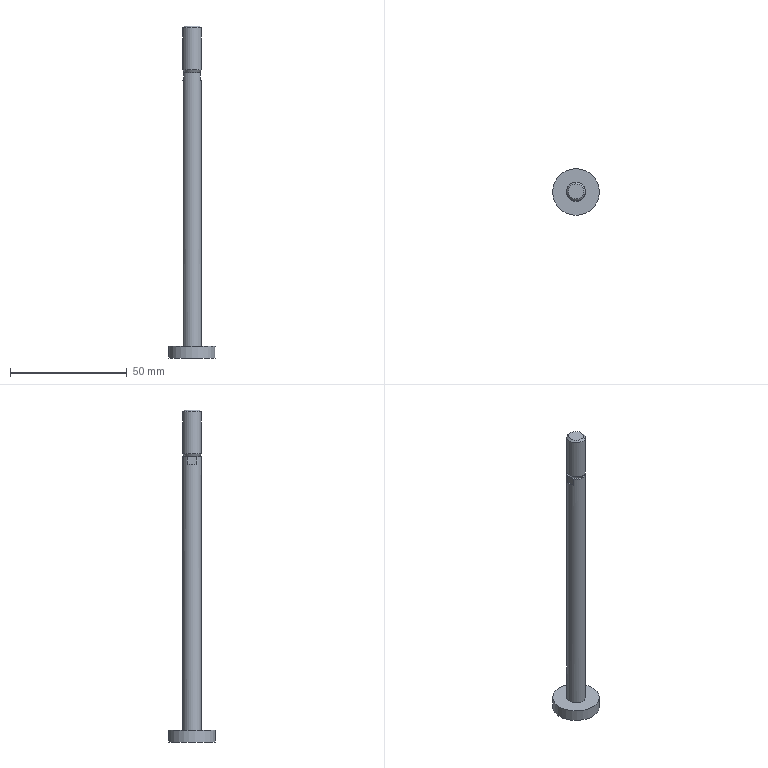Part | STEP file | 1 solid | 13 faces | box 20 x 20 x 142 mm | volume 8430 mm3 | plane 8 | cylinder 3 | cone 2 | commonest cylinder face diameters 8 x2 20 x1
STEP:
#1=CARTESIAN_POINT('',(0.,0.,0.));
#2=DIRECTION('',(0.,0.,1.));
#3=DIRECTION('',(1.,0.,0.));
#4=AXIS2_PLACEMENT_3D('',#1,#2,#3);
#5=CARTESIAN_POINT('',(0.,-3.233,44.));
#6=VERTEX_POINT('',#5);
#7=CARTESIAN_POINT('',(0.,0.,44.));
#8=DIRECTION('',(0.,0.,-1.));
#9=DIRECTION('',(1.,0.,0.));
#10=AXIS2_PLACEMENT_3D('',#7,#8,#9);
#11=CIRCLE('',#10,3.233);
#12=CARTESIAN_POINT('',(0.,0.,43.617));
#13=DIRECTION('',(0.,0.,-1.));
#14=DIRECTION('',(0.,-1.,0.));
#15=AXIS2_PLACEMENT_3D('',#12,#13,#14);
#16=CONICAL_SURFACE('',#15,3.616,0.7854);
#17=CARTESIAN_POINT('',(-1.571,-0.3835));
#18=DIRECTION('',(1.,0.));
#19=VECTOR('',#18,1.);
#20=LINE('',#17,#19);
#21=(GEOMETRIC_REPRESENTATION_CONTEXT(2)PARAMETRIC_REPRESENTATION_CONTEXT()REPRESENTATION_CONTEXT('',''));
#22=DEFINITIONAL_REPRESENTATION('',(#20),#21);
#23=PCURVE('',#16,#22);
#24=CARTESIAN_POINT('',(0.,1.617,44.));
#25=DIRECTION('',(0.,0.,1.));
#26=DIRECTION('',(1.,0.,0.));
#27=AXIS2_PLACEMENT_3D('',#24,#25,#26);
#28=PLANE('',#27);
#29=CARTESIAN_POINT('',(3.233,-1.617));
#30=CARTESIAN_POINT('',(3.233,-7.216));
#31=CARTESIAN_POINT('',(-1.617,-4.416));
#32=CARTESIAN_POINT('',(-6.466,-1.617));
#33=CARTESIAN_POINT('',(-1.617,1.183));
#34=CARTESIAN_POINT('',(3.233,3.983));
#35=CARTESIAN_POINT('',(3.233,-1.617));
#36=(BOUNDED_CURVE()B_SPLINE_CURVE(2,(#29,#30,#31,#32,#33,#34,#35),.UNSPECIFIED.,.T.,.F.)B_SPLINE_CURVE_WITH_KNOTS((1,2,2,2,2,1),(-2.094,0.,2.094,4.189,6.283,8.378),.UNSPECIFIED.)CURVE()GEOMETRIC_REPRESENTATION_ITEM()RATIONAL_B_SPLINE_CURVE((1.,0.5,1.,0.5,1.,0.5,1.))REPRESENTATION_ITEM(''));
#37=(GEOMETRIC_REPRESENTATION_CONTEXT(2)PARAMETRIC_REPRESENTATION_CONTEXT()REPRESENTATION_CONTEXT('',''));
#38=DEFINITIONAL_REPRESENTATION('',(#36),#37);
#39=PCURVE('',#28,#38);
#40=SURFACE_CURVE('',#11,(#23,#39),.PCURVE_S1.);
#41=EDGE_CURVE('',#6,#6,#40,.T.);
#42=ORIENTED_EDGE('',*,*,#41,.T.);
#43=CARTESIAN_POINT('',(0.,-4.,43.233));
#44=VERTEX_POINT('',#43);
#45=CARTESIAN_POINT('',(0.,-3.233,44.));
#46=CARTESIAN_POINT('',(0.,-4.,43.233));
#47=B_SPLINE_CURVE_WITH_KNOTS('',1,(#45,#46),.UNSPECIFIED.,.F.,.F.,(2,2),(-0.5424,0.5424),.PIECEWISE_BEZIER_KNOTS.);
#48=CARTESIAN_POINT('',(6.283,0.));
#49=DIRECTION('',(0.,1.));
#50=VECTOR('',#49,1.);
#51=LINE('',#48,#50);
#52=(GEOMETRIC_REPRESENTATION_CONTEXT(2)PARAMETRIC_REPRESENTATION_CONTEXT()REPRESENTATION_CONTEXT('',''));
#53=DEFINITIONAL_REPRESENTATION('',(#51),#52);
#54=PCURVE('',#16,#53);
#55=CARTESIAN_POINT('',(0.,0.));
#56=DIRECTION('',(0.,1.));
#57=VECTOR('',#56,1.);
#58=LINE('',#55,#57);
#59=(GEOMETRIC_REPRESENTATION_CONTEXT(2)PARAMETRIC_REPRESENTATION_CONTEXT()REPRESENTATION_CONTEXT('',''));
#60=DEFINITIONAL_REPRESENTATION('',(#58),#59);
#61=PCURVE('',#16,#60);
#62=SEAM_CURVE('',#47,(#54,#61),.PCURVE_S1.);
#63=EDGE_CURVE('',#6,#44,#62,.T.);
#64=ORIENTED_EDGE('',*,*,#63,.T.);
#65=CARTESIAN_POINT('',(0.,0.,43.233));
#66=DIRECTION('',(0.,0.,-1.));
#67=DIRECTION('',(1.,0.,0.));
#68=AXIS2_PLACEMENT_3D('',#65,#66,#67);
#69=CIRCLE('',#68,4.);
#70=CARTESIAN_POINT('',(-1.571,0.3835));
#71=DIRECTION('',(1.,0.));
#72=VECTOR('',#71,1.);
#73=LINE('',#70,#72);
#74=(GEOMETRIC_REPRESENTATION_CONTEXT(2)PARAMETRIC_REPRESENTATION_CONTEXT()REPRESENTATION_CONTEXT('',''));
#75=DEFINITIONAL_REPRESENTATION('',(#73),#74);
#76=PCURVE('',#16,#75);
#77=CARTESIAN_POINT('',(0.,0.,34.281));
#78=DIRECTION('',(0.,0.,-1.));
#79=DIRECTION('',(0.,-1.,0.));
#80=AXIS2_PLACEMENT_3D('',#77,#78,#79);
#81=CYLINDRICAL_SURFACE('',#80,4.);
#82=CARTESIAN_POINT('',(-1.571,-8.952));
#83=DIRECTION('',(1.,0.));
#84=VECTOR('',#83,1.);
#85=LINE('',#82,#84);
#86=(GEOMETRIC_REPRESENTATION_CONTEXT(2)PARAMETRIC_REPRESENTATION_CONTEXT()REPRESENTATION_CONTEXT('',''));
#87=DEFINITIONAL_REPRESENTATION('',(#85),#86);
#88=PCURVE('',#81,#87);
#89=SURFACE_CURVE('',#69,(#76,#88),.PCURVE_S1.);
#90=EDGE_CURVE('',#44,#44,#89,.T.);
#91=ORIENTED_EDGE('',*,*,#90,.F.);
#92=ORIENTED_EDGE('',*,*,#63,.F.);
#93=EDGE_LOOP('',(#42,#64,#91,#92));
#94=FACE_BOUND('',#93,.T.);
#95=ADVANCED_FACE('',(#94),#16,.T.);
#96=ORIENTED_EDGE('',*,*,#90,.T.);
#97=CARTESIAN_POINT('',(0.,-4.,25.328));
#98=VERTEX_POINT('',#97);
#99=CARTESIAN_POINT('',(0.,-4.,43.233));
#100=CARTESIAN_POINT('',(0.,-4.,25.328));
#101=B_SPLINE_CURVE_WITH_KNOTS('',1,(#99,#100),.UNSPECIFIED.,.F.,.F.,(2,2),(-8.952,8.952),.PIECEWISE_BEZIER_KNOTS.);
#102=CARTESIAN_POINT('',(6.283,0.));
#103=DIRECTION('',(0.,1.));
#104=VECTOR('',#103,1.);
#105=LINE('',#102,#104);
#106=(GEOMETRIC_REPRESENTATION_CONTEXT(2)PARAMETRIC_REPRESENTATION_CONTEXT()REPRESENTATION_CONTEXT('',''));
#107=DEFINITIONAL_REPRESENTATION('',(#105),#106);
#108=PCURVE('',#81,#107);
#109=CARTESIAN_POINT('',(0.,0.));
#110=DIRECTION('',(0.,1.));
#111=VECTOR('',#110,1.);
#112=LINE('',#109,#111);
#113=(GEOMETRIC_REPRESENTATION_CONTEXT(2)PARAMETRIC_REPRESENTATION_CONTEXT()REPRESENTATION_CONTEXT('',''));
#114=DEFINITIONAL_REPRESENTATION('',(#112),#113);
#115=PCURVE('',#81,#114);
#116=SEAM_CURVE('',#101,(#108,#115),.PCURVE_S1.);
#117=EDGE_CURVE('',#44,#98,#116,.T.);
#118=ORIENTED_EDGE('',*,*,#117,.T.);
#119=CARTESIAN_POINT('',(0.,0.,25.328));
#120=DIRECTION('',(0.,0.,1.));
#121=DIRECTION('',(0.,-1.,0.));
#122=AXIS2_PLACEMENT_3D('',#119,#120,#121);
#123=CIRCLE('',#122,4.);
#124=CARTESIAN_POINT('',(6.283,8.952));
#125=DIRECTION('',(-1.,0.));
#126=VECTOR('',#125,1.);
#127=LINE('',#124,#126);
#128=(GEOMETRIC_REPRESENTATION_CONTEXT(2)PARAMETRIC_REPRESENTATION_CONTEXT()REPRESENTATION_CONTEXT('',''));
#129=DEFINITIONAL_REPRESENTATION('',(#127),#128);
#130=PCURVE('',#81,#129);
#131=CARTESIAN_POINT('',(0.,0.,24.664));
#132=DIRECTION('',(0.,0.,1.));
#133=DIRECTION('',(0.,1.,0.));
#134=AXIS2_PLACEMENT_3D('',#131,#132,#133);
#135=CONICAL_SURFACE('',#134,3.616,0.5236);
#136=CARTESIAN_POINT('',(3.142,0.6642));
#137=DIRECTION('',(1.,0.));
#138=VECTOR('',#137,1.);
#139=LINE('',#136,#138);
#140=(GEOMETRIC_REPRESENTATION_CONTEXT(2)PARAMETRIC_REPRESENTATION_CONTEXT()REPRESENTATION_CONTEXT('',''));
#141=DEFINITIONAL_REPRESENTATION('',(#139),#140);
#142=PCURVE('',#135,#141);
#143=SURFACE_CURVE('',#123,(#130,#142),.PCURVE_S1.);
#144=EDGE_CURVE('',#98,#98,#143,.T.);
#145=ORIENTED_EDGE('',*,*,#144,.T.);
#146=ORIENTED_EDGE('',*,*,#117,.F.);
#147=EDGE_LOOP('',(#96,#118,#145,#146));
#148=FACE_BOUND('',#147,.T.);
#149=ADVANCED_FACE('',(#148),#81,.T.);
#150=ORIENTED_EDGE('',*,*,#41,.F.);
#151=EDGE_LOOP('',(#150));
#152=FACE_BOUND('',#151,.T.);
#153=ADVANCED_FACE('',(#152),#28,.T.);
#154=ORIENTED_EDGE('',*,*,#144,.F.);
#155=CARTESIAN_POINT('',(0.,-3.233,24.));
#156=VERTEX_POINT('',#155);
#157=CARTESIAN_POINT('',(0.,-3.233,24.));
#158=CARTESIAN_POINT('',(0.,-4.,25.328));
#159=B_SPLINE_CURVE_WITH_KNOTS('',1,(#157,#158),.UNSPECIFIED.,.F.,.F.,(2,2),(-0.767,0.767),.PIECEWISE_BEZIER_KNOTS.);
#160=CARTESIAN_POINT('',(3.142,0.));
#161=DIRECTION('',(0.,1.));
#162=VECTOR('',#161,1.);
#163=LINE('',#160,#162);
#164=(GEOMETRIC_REPRESENTATION_CONTEXT(2)PARAMETRIC_REPRESENTATION_CONTEXT()REPRESENTATION_CONTEXT('',''));
#165=DEFINITIONAL_REPRESENTATION('',(#163),#164);
#166=PCURVE('',#135,#165);
#167=CARTESIAN_POINT('',(9.425,0.));
#168=DIRECTION('',(0.,1.));
#169=VECTOR('',#168,1.);
#170=LINE('',#167,#169);
#171=(GEOMETRIC_REPRESENTATION_CONTEXT(2)PARAMETRIC_REPRESENTATION_CONTEXT()REPRESENTATION_CONTEXT('',''));
#172=DEFINITIONAL_REPRESENTATION('',(#170),#171);
#173=PCURVE('',#135,#172);
#174=SEAM_CURVE('',#159,(#166,#173),.PCURVE_S1.);
#175=EDGE_CURVE('',#156,#98,#174,.T.);
#176=ORIENTED_EDGE('',*,*,#175,.F.);
#177=CARTESIAN_POINT('',(0.,0.,24.));
#178=DIRECTION('',(0.,0.,1.));
#179=DIRECTION('',(1.,0.,0.));
#180=AXIS2_PLACEMENT_3D('',#177,#178,#179);
#181=CIRCLE('',#180,3.233);
#182=CARTESIAN_POINT('',(-1.571,-0.6642));
#183=DIRECTION('',(1.,0.));
#184=VECTOR('',#183,1.);
#185=LINE('',#182,#184);
#186=(GEOMETRIC_REPRESENTATION_CONTEXT(2)PARAMETRIC_REPRESENTATION_CONTEXT()REPRESENTATION_CONTEXT('',''));
#187=DEFINITIONAL_REPRESENTATION('',(#185),#186);
#188=PCURVE('',#135,#187);
#189=CARTESIAN_POINT('',(0.,3.616,24.));
#190=DIRECTION('',(0.,0.,1.));
#191=DIRECTION('',(1.,0.,0.));
#192=AXIS2_PLACEMENT_3D('',#189,#190,#191);
#193=PLANE('',#192);
#194=CARTESIAN_POINT('',(0.,-3.616));
#195=DIRECTION('',(1.,0.));
#196=AXIS2_PLACEMENT_2D('',#194,#195);
#197=CIRCLE('',#196,3.233);
#198=(GEOMETRIC_REPRESENTATION_CONTEXT(2)PARAMETRIC_REPRESENTATION_CONTEXT()REPRESENTATION_CONTEXT('',''));
#199=DEFINITIONAL_REPRESENTATION('',(#197),#198);
#200=PCURVE('',#193,#199);
#201=SURFACE_CURVE('',#181,(#188,#200),.PCURVE_S1.);
#202=EDGE_CURVE('',#156,#156,#201,.T.);
#203=ORIENTED_EDGE('',*,*,#202,.T.);
#204=ORIENTED_EDGE('',*,*,#175,.T.);
#205=EDGE_LOOP('',(#154,#176,#203,#204));
#206=FACE_BOUND('',#205,.T.);
#207=ADVANCED_FACE('',(#206),#135,.T.);
#208=CARTESIAN_POINT('',(-3.5,1.936,24.));
#209=VERTEX_POINT('',#208);
#210=CARTESIAN_POINT('',(-3.5,-1.936,24.));
#211=VERTEX_POINT('',#210);
#212=CARTESIAN_POINT('',(-3.5,1.936,24.));
#213=DIRECTION('',(0.,-1.,0.));
#214=VECTOR('',#213,1.);
#215=LINE('',#212,#214);
#216=CARTESIAN_POINT('',(-3.5,-1.68));
#217=DIRECTION('',(0.,-1.));
#218=VECTOR('',#217,1.);
#219=LINE('',#216,#218);
#220=(GEOMETRIC_REPRESENTATION_CONTEXT(2)PARAMETRIC_REPRESENTATION_CONTEXT()REPRESENTATION_CONTEXT('',''));
#221=DEFINITIONAL_REPRESENTATION('',(#219),#220);
#222=PCURVE('',#193,#221);
#223=CARTESIAN_POINT('',(-3.5,20.,24.));
#224=DIRECTION('',(1.,0.,0.));
#225=DIRECTION('',(0.,0.,-1.));
#226=AXIS2_PLACEMENT_3D('',#223,#224,#225);
#227=PLANE('',#226);
#228=CARTESIAN_POINT('',(0.,-18.064));
#229=DIRECTION('',(0.,-1.));
#230=VECTOR('',#229,1.);
#231=LINE('',#228,#230);
#232=(GEOMETRIC_REPRESENTATION_CONTEXT(2)PARAMETRIC_REPRESENTATION_CONTEXT()REPRESENTATION_CONTEXT('',''));
#233=DEFINITIONAL_REPRESENTATION('',(#231),#232);
#234=PCURVE('',#227,#233);
#235=SURFACE_CURVE('',#215,(#222,#234),.PCURVE_S1.);
#236=EDGE_CURVE('',#209,#211,#235,.T.);
#237=ORIENTED_EDGE('',*,*,#236,.T.);
#238=CARTESIAN_POINT('',(0.,-4.,24.));
#239=VERTEX_POINT('',#238);
#240=CARTESIAN_POINT('',(-0.000000002,-0.000000003,24.));
#241=DIRECTION('',(0.,0.,1.));
#242=DIRECTION('',(1.,0.,0.));
#243=AXIS2_PLACEMENT_3D('',#240,#241,#242);
#244=CIRCLE('',#243,4.);
#245=CARTESIAN_POINT('',(-0.000000002,-3.617));
#246=DIRECTION('',(1.,0.));
#247=AXIS2_PLACEMENT_2D('',#245,#246);
#248=CIRCLE('',#247,4.);
#249=(GEOMETRIC_REPRESENTATION_CONTEXT(2)PARAMETRIC_REPRESENTATION_CONTEXT()REPRESENTATION_CONTEXT('',''));
#250=DEFINITIONAL_REPRESENTATION('',(#248),#249);
#251=PCURVE('',#193,#250);
#252=CARTESIAN_POINT('',(0.,0.,-34.5));
#253=DIRECTION('',(0.,0.,-1.));
#254=DIRECTION('',(0.,-1.,0.));
#255=AXIS2_PLACEMENT_3D('',#252,#253,#254);
#256=CYLINDRICAL_SURFACE('',#255,4.);
#257=CARTESIAN_POINT('',(1.065,-58.5));
#258=CARTESIAN_POINT('',(-1.065,-58.5));
#259=B_SPLINE_CURVE_WITH_KNOTS('',1,(#257,#258),.UNSPECIFIED.,.F.,.F.,(2,2),(3.647,5.778),.PIECEWISE_BEZIER_KNOTS.);
#260=(GEOMETRIC_REPRESENTATION_CONTEXT(2)PARAMETRIC_REPRESENTATION_CONTEXT()REPRESENTATION_CONTEXT('',''));
#261=DEFINITIONAL_REPRESENTATION('',(#259),#260);
#262=PCURVE('',#256,#261);
#263=SURFACE_CURVE('',#244,(#251,#262),.PCURVE_S1.);
#264=EDGE_CURVE('',#211,#239,#263,.T.);
#265=ORIENTED_EDGE('',*,*,#264,.T.);
#266=CARTESIAN_POINT('',(3.5,-1.936,24.));
#267=VERTEX_POINT('',#266);
#268=CARTESIAN_POINT('',(-0.000000002,-0.000000003,24.));
#269=DIRECTION('',(0.,0.,1.));
#270=DIRECTION('',(1.,0.,0.));
#271=AXIS2_PLACEMENT_3D('',#268,#269,#270);
#272=CIRCLE('',#271,4.);
#273=CARTESIAN_POINT('',(-0.000000002,-3.617));
#274=DIRECTION('',(1.,0.));
#275=AXIS2_PLACEMENT_2D('',#273,#274);
#276=CIRCLE('',#275,4.);
#277=(GEOMETRIC_REPRESENTATION_CONTEXT(2)PARAMETRIC_REPRESENTATION_CONTEXT()REPRESENTATION_CONTEXT('',''));
#278=DEFINITIONAL_REPRESENTATION('',(#276),#277);
#279=PCURVE('',#193,#278);
#280=CARTESIAN_POINT('',(7.349,-58.5));
#281=CARTESIAN_POINT('',(5.218,-58.5));
#282=B_SPLINE_CURVE_WITH_KNOTS('',1,(#280,#281),.UNSPECIFIED.,.F.,.F.,(2,2),(3.647,5.778),.PIECEWISE_BEZIER_KNOTS.);
#283=(GEOMETRIC_REPRESENTATION_CONTEXT(2)PARAMETRIC_REPRESENTATION_CONTEXT()REPRESENTATION_CONTEXT('',''));
#284=DEFINITIONAL_REPRESENTATION('',(#282),#283);
#285=PCURVE('',#256,#284);
#286=SURFACE_CURVE('',#272,(#279,#285),.PCURVE_S1.);
#287=EDGE_CURVE('',#239,#267,#286,.T.);
#288=ORIENTED_EDGE('',*,*,#287,.T.);
#289=CARTESIAN_POINT('',(3.5,1.936,24.));
#290=VERTEX_POINT('',#289);
#291=CARTESIAN_POINT('',(3.5,-1.936,24.));
#292=DIRECTION('',(0.,1.,0.));
#293=VECTOR('',#292,1.);
#294=LINE('',#291,#293);
#295=CARTESIAN_POINT('',(3.5,-5.553));
#296=DIRECTION('',(0.,1.));
#297=VECTOR('',#296,1.);
#298=LINE('',#295,#297);
#299=(GEOMETRIC_REPRESENTATION_CONTEXT(2)PARAMETRIC_REPRESENTATION_CONTEXT()REPRESENTATION_CONTEXT('',''));
#300=DEFINITIONAL_REPRESENTATION('',(#298),#299);
#301=PCURVE('',#193,#300);
#302=CARTESIAN_POINT('',(3.5,20.,20.8));
#303=DIRECTION('',(-1.,0.,0.));
#304=DIRECTION('',(0.,0.,1.));
#305=AXIS2_PLACEMENT_3D('',#302,#303,#304);
#306=PLANE('',#305);
#307=CARTESIAN_POINT('',(3.2,-21.936));
#308=DIRECTION('',(0.,1.));
#309=VECTOR('',#308,1.);
#310=LINE('',#307,#309);
#311=(GEOMETRIC_REPRESENTATION_CONTEXT(2)PARAMETRIC_REPRESENTATION_CONTEXT()REPRESENTATION_CONTEXT('',''));
#312=DEFINITIONAL_REPRESENTATION('',(#310),#311);
#313=PCURVE('',#306,#312);
#314=SURFACE_CURVE('',#294,(#301,#313),.PCURVE_S1.);
#315=EDGE_CURVE('',#267,#290,#314,.T.);
#316=ORIENTED_EDGE('',*,*,#315,.T.);
#317=CARTESIAN_POINT('',(-0.000000003,-0.000000003,24.));
#318=DIRECTION('',(0.,0.,1.));
#319=DIRECTION('',(1.,0.,0.));
#320=AXIS2_PLACEMENT_3D('',#317,#318,#319);
#321=CIRCLE('',#320,4.);
#322=CARTESIAN_POINT('',(-0.000000003,-3.617));
#323=DIRECTION('',(1.,0.));
#324=AXIS2_PLACEMENT_2D('',#322,#323);
#325=CIRCLE('',#324,4.);
#326=(GEOMETRIC_REPRESENTATION_CONTEXT(2)PARAMETRIC_REPRESENTATION_CONTEXT()REPRESENTATION_CONTEXT('',''));
#327=DEFINITIONAL_REPRESENTATION('',(#325),#326);
#328=PCURVE('',#193,#327);
#329=CARTESIAN_POINT('',(4.207,-58.5));
#330=CARTESIAN_POINT('',(2.076,-58.5));
#331=B_SPLINE_CURVE_WITH_KNOTS('',1,(#329,#330),.UNSPECIFIED.,.F.,.F.,(2,2),(0.5054,2.636),.PIECEWISE_BEZIER_KNOTS.);
#332=(GEOMETRIC_REPRESENTATION_CONTEXT(2)PARAMETRIC_REPRESENTATION_CONTEXT()REPRESENTATION_CONTEXT('',''));
#333=DEFINITIONAL_REPRESENTATION('',(#331),#332);
#334=PCURVE('',#256,#333);
#335=SURFACE_CURVE('',#321,(#328,#334),.PCURVE_S1.);
#336=EDGE_CURVE('',#290,#209,#335,.T.);
#337=ORIENTED_EDGE('',*,*,#336,.T.);
#338=EDGE_LOOP('',(#237,#265,#288,#316,#337));
#339=FACE_BOUND('',#338,.T.);
#340=ORIENTED_EDGE('',*,*,#202,.F.);
#341=EDGE_LOOP('',(#340));
#342=FACE_BOUND('',#341,.T.);
#343=ADVANCED_FACE('',(#339,#342),#193,.T.);
#344=CARTESIAN_POINT('',(-3.5,-1.936,20.8));
#345=VERTEX_POINT('',#344);
#346=CARTESIAN_POINT('',(-3.5,-1.936,24.));
#347=DIRECTION('',(0.,0.,-1.));
#348=VECTOR('',#347,1.);
#349=LINE('',#346,#348);
#350=CARTESIAN_POINT('',(0.,-21.936));
#351=DIRECTION('',(1.,0.));
#352=VECTOR('',#351,1.);
#353=LINE('',#350,#352);
#354=(GEOMETRIC_REPRESENTATION_CONTEXT(2)PARAMETRIC_REPRESENTATION_CONTEXT()REPRESENTATION_CONTEXT('',''));
#355=DEFINITIONAL_REPRESENTATION('',(#353),#354);
#356=PCURVE('',#227,#355);
#357=CARTESIAN_POINT('',(1.065,-58.5));
#358=DIRECTION('',(0.,1.));
#359=VECTOR('',#358,1.);
#360=LINE('',#357,#359);
#361=(GEOMETRIC_REPRESENTATION_CONTEXT(2)PARAMETRIC_REPRESENTATION_CONTEXT()REPRESENTATION_CONTEXT('',''));
#362=DEFINITIONAL_REPRESENTATION('',(#360),#361);
#363=PCURVE('',#256,#362);
#364=SURFACE_CURVE('',#349,(#356,#363),.PCURVE_S1.);
#365=EDGE_CURVE('',#211,#345,#364,.T.);
#366=ORIENTED_EDGE('',*,*,#365,.F.);
#367=ORIENTED_EDGE('',*,*,#236,.F.);
#368=CARTESIAN_POINT('',(-3.5,1.936,20.8));
#369=VERTEX_POINT('',#368);
#370=CARTESIAN_POINT('',(-3.5,1.936,20.8));
#371=DIRECTION('',(0.,0.,1.));
#372=VECTOR('',#371,1.);
#373=LINE('',#370,#372);
#374=CARTESIAN_POINT('',(3.2,-18.064));
#375=DIRECTION('',(-1.,0.));
#376=VECTOR('',#375,1.);
#377=LINE('',#374,#376);
#378=(GEOMETRIC_REPRESENTATION_CONTEXT(2)PARAMETRIC_REPRESENTATION_CONTEXT()REPRESENTATION_CONTEXT('',''));
#379=DEFINITIONAL_REPRESENTATION('',(#377),#378);
#380=PCURVE('',#227,#379);
#381=CARTESIAN_POINT('',(2.076,-55.3));
#382=DIRECTION('',(0.,-1.));
#383=VECTOR('',#382,1.);
#384=LINE('',#381,#383);
#385=(GEOMETRIC_REPRESENTATION_CONTEXT(2)PARAMETRIC_REPRESENTATION_CONTEXT()REPRESENTATION_CONTEXT('',''));
#386=DEFINITIONAL_REPRESENTATION('',(#384),#385);
#387=PCURVE('',#256,#386);
#388=SURFACE_CURVE('',#373,(#380,#387),.PCURVE_S1.);
#389=EDGE_CURVE('',#369,#209,#388,.T.);
#390=ORIENTED_EDGE('',*,*,#389,.F.);
#391=CARTESIAN_POINT('',(-3.5,1.936,20.8));
#392=DIRECTION('',(0.,-1.,0.));
#393=VECTOR('',#392,1.);
#394=LINE('',#391,#393);
#395=CARTESIAN_POINT('',(3.2,-18.064));
#396=DIRECTION('',(0.,-1.));
#397=VECTOR('',#396,1.);
#398=LINE('',#395,#397);
#399=(GEOMETRIC_REPRESENTATION_CONTEXT(2)PARAMETRIC_REPRESENTATION_CONTEXT()REPRESENTATION_CONTEXT('',''));
#400=DEFINITIONAL_REPRESENTATION('',(#398),#399);
#401=PCURVE('',#227,#400);
#402=CARTESIAN_POINT('',(-3.5,20.,20.8));
#403=DIRECTION('',(0.,0.,-1.));
#404=DIRECTION('',(-1.,0.,0.));
#405=AXIS2_PLACEMENT_3D('',#402,#403,#404);
#406=PLANE('',#405);
#407=CARTESIAN_POINT('',(0.,-18.064));
#408=DIRECTION('',(0.,-1.));
#409=VECTOR('',#408,1.);
#410=LINE('',#407,#409);
#411=(GEOMETRIC_REPRESENTATION_CONTEXT(2)PARAMETRIC_REPRESENTATION_CONTEXT()REPRESENTATION_CONTEXT('',''));
#412=DEFINITIONAL_REPRESENTATION('',(#410),#411);
#413=PCURVE('',#406,#412);
#414=SURFACE_CURVE('',#394,(#401,#413),.PCURVE_S1.);
#415=EDGE_CURVE('',#369,#345,#414,.T.);
#416=ORIENTED_EDGE('',*,*,#415,.T.);
#417=EDGE_LOOP('',(#366,#367,#390,#416));
#418=FACE_BOUND('',#417,.T.);
#419=ADVANCED_FACE('',(#418),#227,.F.);
#420=ORIENTED_EDGE('',*,*,#287,.F.);
#421=CARTESIAN_POINT('',(0.,-4.,-93.));
#422=VERTEX_POINT('',#421);
#423=CARTESIAN_POINT('',(0.,-4.,24.));
#424=CARTESIAN_POINT('',(0.,-4.,-93.));
#425=B_SPLINE_CURVE_WITH_KNOTS('',1,(#423,#424),.UNSPECIFIED.,.F.,.F.,(2,2),(-58.5,58.5),.PIECEWISE_BEZIER_KNOTS.);
#426=CARTESIAN_POINT('',(6.283,0.));
#427=DIRECTION('',(0.,1.));
#428=VECTOR('',#427,1.);
#429=LINE('',#426,#428);
#430=(GEOMETRIC_REPRESENTATION_CONTEXT(2)PARAMETRIC_REPRESENTATION_CONTEXT()REPRESENTATION_CONTEXT('',''));
#431=DEFINITIONAL_REPRESENTATION('',(#429),#430);
#432=PCURVE('',#256,#431);
#433=CARTESIAN_POINT('',(0.,0.));
#434=DIRECTION('',(0.,1.));
#435=VECTOR('',#434,1.);
#436=LINE('',#433,#435);
#437=(GEOMETRIC_REPRESENTATION_CONTEXT(2)PARAMETRIC_REPRESENTATION_CONTEXT()REPRESENTATION_CONTEXT('',''));
#438=DEFINITIONAL_REPRESENTATION('',(#436),#437);
#439=PCURVE('',#256,#438);
#440=SEAM_CURVE('',#425,(#432,#439),.PCURVE_S1.);
#441=EDGE_CURVE('',#239,#422,#440,.T.);
#442=ORIENTED_EDGE('',*,*,#441,.T.);
#443=CARTESIAN_POINT('',(0.,0.,-93.));
#444=DIRECTION('',(0.,0.,-1.));
#445=DIRECTION('',(1.,0.,0.));
#446=AXIS2_PLACEMENT_3D('',#443,#444,#445);
#447=CIRCLE('',#446,4.);
#448=CARTESIAN_POINT('',(-1.571,58.5));
#449=DIRECTION('',(1.,0.));
#450=VECTOR('',#449,1.);
#451=LINE('',#448,#450);
#452=(GEOMETRIC_REPRESENTATION_CONTEXT(2)PARAMETRIC_REPRESENTATION_CONTEXT()REPRESENTATION_CONTEXT('',''));
#453=DEFINITIONAL_REPRESENTATION('',(#451),#452);
#454=PCURVE('',#256,#453);
#455=CARTESIAN_POINT('',(0.,7.,-93.));
#456=DIRECTION('',(0.,0.,1.));
#457=DIRECTION('',(1.,0.,0.));
#458=AXIS2_PLACEMENT_3D('',#455,#456,#457);
#459=PLANE('',#458);
#460=CARTESIAN_POINT('',(4.,-7.));
#461=CARTESIAN_POINT('',(4.,-13.928));
#462=CARTESIAN_POINT('',(-2.,-10.464));
#463=CARTESIAN_POINT('',(-8.,-7.));
#464=CARTESIAN_POINT('',(-2.,-3.536));
#465=CARTESIAN_POINT('',(4.,-0.0718));
#466=CARTESIAN_POINT('',(4.,-7.));
#467=(BOUNDED_CURVE()B_SPLINE_CURVE(2,(#460,#461,#462,#463,#464,#465,#466),.UNSPECIFIED.,.T.,.F.)B_SPLINE_CURVE_WITH_KNOTS((1,2,2,2,2,1),(-2.094,0.,2.094,4.189,6.283,8.378),.UNSPECIFIED.)CURVE()GEOMETRIC_REPRESENTATION_ITEM()RATIONAL_B_SPLINE_CURVE((1.,0.5,1.,0.5,1.,0.5,1.))REPRESENTATION_ITEM(''));
#468=(GEOMETRIC_REPRESENTATION_CONTEXT(2)PARAMETRIC_REPRESENTATION_CONTEXT()REPRESENTATION_CONTEXT('',''));
#469=DEFINITIONAL_REPRESENTATION('',(#467),#468);
#470=PCURVE('',#459,#469);
#471=SURFACE_CURVE('',#447,(#454,#470),.PCURVE_S1.);
#472=EDGE_CURVE('',#422,#422,#471,.T.);
#473=ORIENTED_EDGE('',*,*,#472,.F.);
#474=ORIENTED_EDGE('',*,*,#441,.F.);
#475=ORIENTED_EDGE('',*,*,#264,.F.);
#476=ORIENTED_EDGE('',*,*,#365,.T.);
#477=CARTESIAN_POINT('',(0.,0.,20.8));
#478=DIRECTION('',(0.,0.,-1.));
#479=DIRECTION('',(1.,0.,0.));
#480=AXIS2_PLACEMENT_3D('',#477,#478,#479);
#481=CIRCLE('',#480,4.);
#482=CARTESIAN_POINT('',(-1.571,-55.3));
#483=DIRECTION('',(1.,0.));
#484=VECTOR('',#483,1.);
#485=LINE('',#482,#484);
#486=(GEOMETRIC_REPRESENTATION_CONTEXT(2)PARAMETRIC_REPRESENTATION_CONTEXT()REPRESENTATION_CONTEXT('',''));
#487=DEFINITIONAL_REPRESENTATION('',(#485),#486);
#488=PCURVE('',#256,#487);
#489=CARTESIAN_POINT('',(-3.5,-20.));
#490=DIRECTION('',(-1.,0.));
#491=AXIS2_PLACEMENT_2D('',#489,#490);
#492=CIRCLE('',#491,4.);
#493=(GEOMETRIC_REPRESENTATION_CONTEXT(2)PARAMETRIC_REPRESENTATION_CONTEXT()REPRESENTATION_CONTEXT('',''));
#494=DEFINITIONAL_REPRESENTATION('',(#492),#493);
#495=PCURVE('',#406,#494);
#496=SURFACE_CURVE('',#481,(#488,#495),.PCURVE_S1.);
#497=EDGE_CURVE('',#345,#369,#496,.T.);
#498=ORIENTED_EDGE('',*,*,#497,.T.);
#499=ORIENTED_EDGE('',*,*,#389,.T.);
#500=ORIENTED_EDGE('',*,*,#336,.F.);
#501=CARTESIAN_POINT('',(3.5,1.936,20.8));
#502=VERTEX_POINT('',#501);
#503=CARTESIAN_POINT('',(3.5,1.936,24.));
#504=DIRECTION('',(0.,0.,-1.));
#505=VECTOR('',#504,1.);
#506=LINE('',#503,#505);
#507=CARTESIAN_POINT('',(4.207,-58.5));
#508=DIRECTION('',(0.,1.));
#509=VECTOR('',#508,1.);
#510=LINE('',#507,#509);
#511=(GEOMETRIC_REPRESENTATION_CONTEXT(2)PARAMETRIC_REPRESENTATION_CONTEXT()REPRESENTATION_CONTEXT('',''));
#512=DEFINITIONAL_REPRESENTATION('',(#510),#511);
#513=PCURVE('',#256,#512);
#514=CARTESIAN_POINT('',(3.2,-18.064));
#515=DIRECTION('',(-1.,0.));
#516=VECTOR('',#515,1.);
#517=LINE('',#514,#516);
#518=(GEOMETRIC_REPRESENTATION_CONTEXT(2)PARAMETRIC_REPRESENTATION_CONTEXT()REPRESENTATION_CONTEXT('',''));
#519=DEFINITIONAL_REPRESENTATION('',(#517),#518);
#520=PCURVE('',#306,#519);
#521=SURFACE_CURVE('',#506,(#513,#520),.PCURVE_S1.);
#522=EDGE_CURVE('',#290,#502,#521,.T.);
#523=ORIENTED_EDGE('',*,*,#522,.T.);
#524=CARTESIAN_POINT('',(3.5,-1.936,20.8));
#525=VERTEX_POINT('',#524);
#526=CARTESIAN_POINT('',(0.,0.,20.8));
#527=DIRECTION('',(0.,0.,-1.));
#528=DIRECTION('',(1.,0.,0.));
#529=AXIS2_PLACEMENT_3D('',#526,#527,#528);
#530=CIRCLE('',#529,4.);
#531=CARTESIAN_POINT('',(-1.571,-55.3));
#532=DIRECTION('',(1.,0.));
#533=VECTOR('',#532,1.);
#534=LINE('',#531,#533);
#535=(GEOMETRIC_REPRESENTATION_CONTEXT(2)PARAMETRIC_REPRESENTATION_CONTEXT()REPRESENTATION_CONTEXT('',''));
#536=DEFINITIONAL_REPRESENTATION('',(#534),#535);
#537=PCURVE('',#256,#536);
#538=CARTESIAN_POINT('',(13.5,20.,20.8));
#539=DIRECTION('',(0.,0.,-1.));
#540=DIRECTION('',(-1.,0.,0.));
#541=AXIS2_PLACEMENT_3D('',#538,#539,#540);
#542=PLANE('',#541);
#543=CARTESIAN_POINT('',(13.5,-20.));
#544=DIRECTION('',(-1.,0.));
#545=AXIS2_PLACEMENT_2D('',#543,#544);
#546=CIRCLE('',#545,4.);
#547=(GEOMETRIC_REPRESENTATION_CONTEXT(2)PARAMETRIC_REPRESENTATION_CONTEXT()REPRESENTATION_CONTEXT('',''));
#548=DEFINITIONAL_REPRESENTATION('',(#546),#547);
#549=PCURVE('',#542,#548);
#550=SURFACE_CURVE('',#530,(#537,#549),.PCURVE_S1.);
#551=EDGE_CURVE('',#502,#525,#550,.T.);
#552=ORIENTED_EDGE('',*,*,#551,.T.);
#553=CARTESIAN_POINT('',(3.5,-1.936,24.));
#554=DIRECTION('',(0.,0.,-1.));
#555=VECTOR('',#554,1.);
#556=LINE('',#553,#555);
#557=CARTESIAN_POINT('',(5.218,-58.5));
#558=DIRECTION('',(0.,1.));
#559=VECTOR('',#558,1.);
#560=LINE('',#557,#559);
#561=(GEOMETRIC_REPRESENTATION_CONTEXT(2)PARAMETRIC_REPRESENTATION_CONTEXT()REPRESENTATION_CONTEXT('',''));
#562=DEFINITIONAL_REPRESENTATION('',(#560),#561);
#563=PCURVE('',#256,#562);
#564=CARTESIAN_POINT('',(3.2,-21.936));
#565=DIRECTION('',(-1.,0.));
#566=VECTOR('',#565,1.);
#567=LINE('',#564,#566);
#568=(GEOMETRIC_REPRESENTATION_CONTEXT(2)PARAMETRIC_REPRESENTATION_CONTEXT()REPRESENTATION_CONTEXT('',''));
#569=DEFINITIONAL_REPRESENTATION('',(#567),#568);
#570=PCURVE('',#306,#569);
#571=SURFACE_CURVE('',#556,(#563,#570),.PCURVE_S1.);
#572=EDGE_CURVE('',#267,#525,#571,.T.);
#573=ORIENTED_EDGE('',*,*,#572,.F.);
#574=EDGE_LOOP('',(#420,#442,#473,#474,#475,#476,#498,#499,#500,#523,#552,#573));
#575=FACE_BOUND('',#574,.T.);
#576=ADVANCED_FACE('',(#575),#256,.T.);
#577=ORIENTED_EDGE('',*,*,#572,.T.);
#578=CARTESIAN_POINT('',(3.5,1.936,20.8));
#579=DIRECTION('',(0.,-1.,0.));
#580=VECTOR('',#579,1.);
#581=LINE('',#578,#580);
#582=CARTESIAN_POINT('',(0.,-18.064));
#583=DIRECTION('',(0.,-1.));
#584=VECTOR('',#583,1.);
#585=LINE('',#582,#584);
#586=(GEOMETRIC_REPRESENTATION_CONTEXT(2)PARAMETRIC_REPRESENTATION_CONTEXT()REPRESENTATION_CONTEXT('',''));
#587=DEFINITIONAL_REPRESENTATION('',(#585),#586);
#588=PCURVE('',#306,#587);
#589=CARTESIAN_POINT('',(10.,-18.064));
#590=DIRECTION('',(0.,-1.));
#591=VECTOR('',#590,1.);
#592=LINE('',#589,#591);
#593=(GEOMETRIC_REPRESENTATION_CONTEXT(2)PARAMETRIC_REPRESENTATION_CONTEXT()REPRESENTATION_CONTEXT('',''));
#594=DEFINITIONAL_REPRESENTATION('',(#592),#593);
#595=PCURVE('',#542,#594);
#596=SURFACE_CURVE('',#581,(#588,#595),.PCURVE_S1.);
#597=EDGE_CURVE('',#502,#525,#596,.T.);
#598=ORIENTED_EDGE('',*,*,#597,.F.);
#599=ORIENTED_EDGE('',*,*,#522,.F.);
#600=ORIENTED_EDGE('',*,*,#315,.F.);
#601=EDGE_LOOP('',(#577,#598,#599,#600));
#602=FACE_BOUND('',#601,.T.);
#603=ADVANCED_FACE('',(#602),#306,.F.);
#604=ORIENTED_EDGE('',*,*,#497,.F.);
#605=ORIENTED_EDGE('',*,*,#415,.F.);
#606=EDGE_LOOP('',(#604,#605));
#607=FACE_BOUND('',#606,.T.);
#608=ADVANCED_FACE('',(#607),#406,.F.);
#609=CARTESIAN_POINT('',(0.,-10.,-93.));
#610=VERTEX_POINT('',#609);
#611=CARTESIAN_POINT('',(0.,0.,-93.));
#612=DIRECTION('',(0.,0.,1.));
#613=DIRECTION('',(1.,0.,0.));
#614=AXIS2_PLACEMENT_3D('',#611,#612,#613);
#615=CIRCLE('',#614,10.);
#616=CARTESIAN_POINT('',(0.,-7.));
#617=DIRECTION('',(1.,0.));
#618=AXIS2_PLACEMENT_2D('',#616,#617);
#619=CIRCLE('',#618,10.);
#620=(GEOMETRIC_REPRESENTATION_CONTEXT(2)PARAMETRIC_REPRESENTATION_CONTEXT()REPRESENTATION_CONTEXT('',''));
#621=DEFINITIONAL_REPRESENTATION('',(#619),#620);
#622=PCURVE('',#459,#621);
#623=CARTESIAN_POINT('',(0.,0.,-95.5));
#624=DIRECTION('',(0.,0.,-1.));
#625=DIRECTION('',(0.,-1.,0.));
#626=AXIS2_PLACEMENT_3D('',#623,#624,#625);
#627=CYLINDRICAL_SURFACE('',#626,10.);
#628=CARTESIAN_POINT('',(10.996,-2.5));
#629=DIRECTION('',(-1.,0.));
#630=VECTOR('',#629,1.);
#631=LINE('',#628,#630);
#632=(GEOMETRIC_REPRESENTATION_CONTEXT(2)PARAMETRIC_REPRESENTATION_CONTEXT()REPRESENTATION_CONTEXT('',''));
#633=DEFINITIONAL_REPRESENTATION('',(#631),#632);
#634=PCURVE('',#627,#633);
#635=SURFACE_CURVE('',#615,(#622,#634),.PCURVE_S1.);
#636=EDGE_CURVE('',#610,#610,#635,.T.);
#637=ORIENTED_EDGE('',*,*,#636,.T.);
#638=EDGE_LOOP('',(#637));
#639=FACE_BOUND('',#638,.T.);
#640=ORIENTED_EDGE('',*,*,#472,.T.);
#641=EDGE_LOOP('',(#640));
#642=FACE_BOUND('',#641,.T.);
#643=ADVANCED_FACE('',(#639,#642),#459,.T.);
#644=ORIENTED_EDGE('',*,*,#551,.F.);
#645=ORIENTED_EDGE('',*,*,#597,.T.);
#646=EDGE_LOOP('',(#644,#645));
#647=FACE_BOUND('',#646,.T.);
#648=ADVANCED_FACE('',(#647),#542,.F.);
#649=ORIENTED_EDGE('',*,*,#636,.F.);
#650=CARTESIAN_POINT('',(0.,-10.,-98.));
#651=VERTEX_POINT('',#650);
#652=CARTESIAN_POINT('',(0.,-10.,-93.));
#653=CARTESIAN_POINT('',(0.,-10.,-98.));
#654=B_SPLINE_CURVE_WITH_KNOTS('',1,(#652,#653),.UNSPECIFIED.,.F.,.F.,(2,2),(-2.5,2.5),.PIECEWISE_BEZIER_KNOTS.);
#655=CARTESIAN_POINT('',(6.283,0.));
#656=DIRECTION('',(0.,1.));
#657=VECTOR('',#656,1.);
#658=LINE('',#655,#657);
#659=(GEOMETRIC_REPRESENTATION_CONTEXT(2)PARAMETRIC_REPRESENTATION_CONTEXT()REPRESENTATION_CONTEXT('',''));
#660=DEFINITIONAL_REPRESENTATION('',(#658),#659);
#661=PCURVE('',#627,#660);
#662=CARTESIAN_POINT('',(0.,0.));
#663=DIRECTION('',(0.,1.));
#664=VECTOR('',#663,1.);
#665=LINE('',#662,#664);
#666=(GEOMETRIC_REPRESENTATION_CONTEXT(2)PARAMETRIC_REPRESENTATION_CONTEXT()REPRESENTATION_CONTEXT('',''));
#667=DEFINITIONAL_REPRESENTATION('',(#665),#666);
#668=PCURVE('',#627,#667);
#669=SEAM_CURVE('',#654,(#661,#668),.PCURVE_S1.);
#670=EDGE_CURVE('',#610,#651,#669,.T.);
#671=ORIENTED_EDGE('',*,*,#670,.T.);
#672=CARTESIAN_POINT('',(0.,0.,-98.));
#673=DIRECTION('',(0.,0.,-1.));
#674=DIRECTION('',(1.,0.,0.));
#675=AXIS2_PLACEMENT_3D('',#672,#673,#674);
#676=CIRCLE('',#675,10.);
#677=CARTESIAN_POINT('',(-1.571,2.5));
#678=DIRECTION('',(1.,0.));
#679=VECTOR('',#678,1.);
#680=LINE('',#677,#679);
#681=(GEOMETRIC_REPRESENTATION_CONTEXT(2)PARAMETRIC_REPRESENTATION_CONTEXT()REPRESENTATION_CONTEXT('',''));
#682=DEFINITIONAL_REPRESENTATION('',(#680),#681);
#683=PCURVE('',#627,#682);
#684=CARTESIAN_POINT('',(0.,5.,-98.));
#685=DIRECTION('',(0.,0.,-1.));
#686=DIRECTION('',(-1.,0.,0.));
#687=AXIS2_PLACEMENT_3D('',#684,#685,#686);
#688=PLANE('',#687);
#689=CARTESIAN_POINT('',(0.,-5.));
#690=DIRECTION('',(-1.,0.));
#691=AXIS2_PLACEMENT_2D('',#689,#690);
#692=CIRCLE('',#691,10.);
#693=(GEOMETRIC_REPRESENTATION_CONTEXT(2)PARAMETRIC_REPRESENTATION_CONTEXT()REPRESENTATION_CONTEXT('',''));
#694=DEFINITIONAL_REPRESENTATION('',(#692),#693);
#695=PCURVE('',#688,#694);
#696=SURFACE_CURVE('',#676,(#683,#695),.PCURVE_S1.);
#697=EDGE_CURVE('',#651,#651,#696,.T.);
#698=ORIENTED_EDGE('',*,*,#697,.F.);
#699=ORIENTED_EDGE('',*,*,#670,.F.);
#700=EDGE_LOOP('',(#649,#671,#698,#699));
#701=FACE_BOUND('',#700,.T.);
#702=ADVANCED_FACE('',(#701),#627,.T.);
#703=ORIENTED_EDGE('',*,*,#697,.T.);
#704=EDGE_LOOP('',(#703));
#705=FACE_BOUND('',#704,.T.);
#706=ADVANCED_FACE('',(#705),#688,.T.);
#707=CLOSED_SHELL('',(#95,#149,#153,#207,#343,#419,#576,#603,#608,#643,#648,#702,#706));
#708=MANIFOLD_SOLID_BREP('',#707);
#709=(LENGTH_UNIT()NAMED_UNIT(*)SI_UNIT(.MILLI.,.METRE.));
#710=UNCERTAINTY_MEASURE_WITH_UNIT(LENGTH_MEASURE(0.000005),#709,'','');
#711=(NAMED_UNIT(*)PLANE_ANGLE_UNIT()SI_UNIT($,.RADIAN.));
#712=(NAMED_UNIT(*)SI_UNIT($,.STERADIAN.)SOLID_ANGLE_UNIT());
#713=(GEOMETRIC_REPRESENTATION_CONTEXT(3)GLOBAL_UNCERTAINTY_ASSIGNED_CONTEXT((#710))GLOBAL_UNIT_ASSIGNED_CONTEXT((#709,#711,#712))REPRESENTATION_CONTEXT('',''));
#714=ADVANCED_BREP_SHAPE_REPRESENTATION('',(#4,#708),#713);